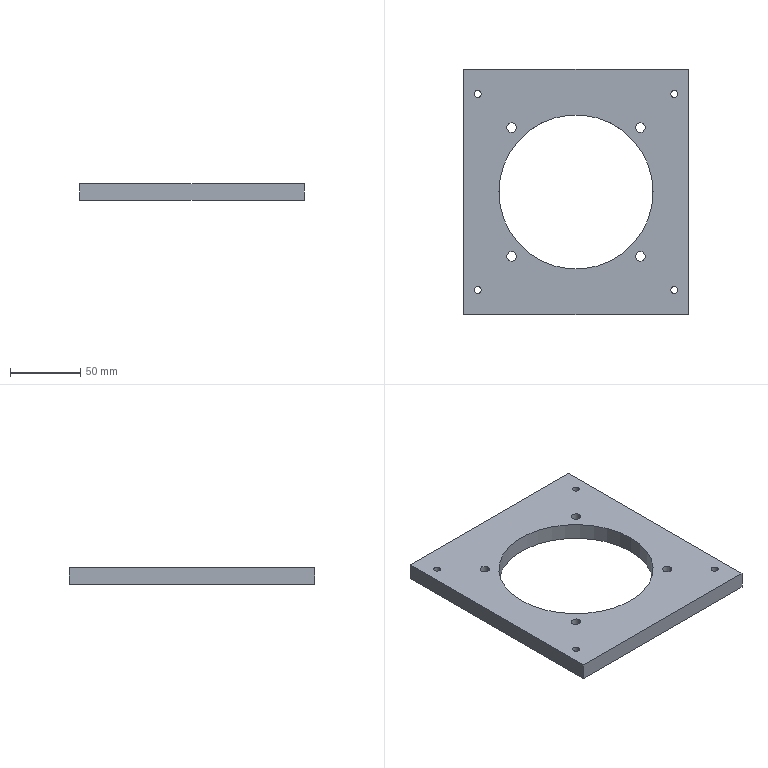Part | STEP file | PN_0003_motor mounting plate_default_machined_ | 1 solid | 24 faces | box 160 x 175 x 12 mm | volume 219275 mm3 | cylinder 18 | plane 6 | commonest cylinder face diameters 5 x8 6.8 x8 110 x2